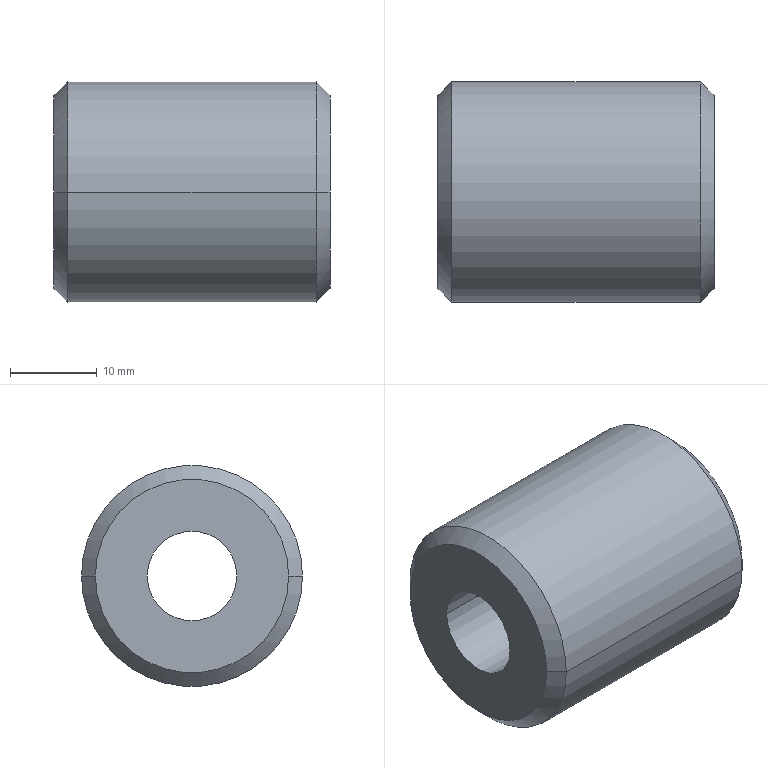Part | NX | features BREP 1 | 1 solid | 10 faces | box 31.75 x 25.4 x 25.4 mm | volume 13243 mm3 | cone 4 | cylinder 4 | plane 2 | commonest cylinder face diameters 10.312 x2 25.4 x2
STEP:
#1=CARTESIAN_POINT('',(-15.875,11.113,0.));
#2=VERTEX_POINT('',#1);
#3=CARTESIAN_POINT('',(-15.875,-11.113,0.));
#4=VERTEX_POINT('',#3);
#5=CARTESIAN_POINT('',(-15.875,0.,0.));
#6=DIRECTION('',(1.,0.,0.));
#7=DIRECTION('',(0.,1.,0.));
#8=AXIS2_PLACEMENT_3D('',#5,#6,#7);
#9=CIRCLE('',#8,11.113);
#10=EDGE_CURVE('',#2,#4,#9,.T.);
#11=ORIENTED_EDGE('',*,*,#10,.F.);
#12=CARTESIAN_POINT('',(-15.875,0.,0.));
#13=DIRECTION('',(1.,0.,0.));
#14=DIRECTION('',(0.,-1.,0.));
#15=AXIS2_PLACEMENT_3D('',#12,#13,#14);
#16=CIRCLE('',#15,11.113);
#17=EDGE_CURVE('',#4,#2,#16,.T.);
#18=ORIENTED_EDGE('',*,*,#17,.F.);
#19=EDGE_LOOP('',(#11,#18));
#20=FACE_BOUND('',#19,.T.);
#21=CARTESIAN_POINT('',(-15.875,5.156,0.));
#22=VERTEX_POINT('',#21);
#23=CARTESIAN_POINT('',(-15.875,-5.156,0.));
#24=VERTEX_POINT('',#23);
#25=CARTESIAN_POINT('',(-15.875,0.,0.));
#26=DIRECTION('',(-1.,0.,0.));
#27=DIRECTION('',(0.,1.,0.));
#28=AXIS2_PLACEMENT_3D('',#25,#26,#27);
#29=CIRCLE('',#28,5.156);
#30=EDGE_CURVE('',#22,#24,#29,.T.);
#31=ORIENTED_EDGE('',*,*,#30,.F.);
#32=CARTESIAN_POINT('',(-15.875,0.,0.));
#33=DIRECTION('',(-1.,0.,0.));
#34=DIRECTION('',(0.,-1.,0.));
#35=AXIS2_PLACEMENT_3D('',#32,#33,#34);
#36=CIRCLE('',#35,5.156);
#37=EDGE_CURVE('',#24,#22,#36,.T.);
#38=ORIENTED_EDGE('',*,*,#37,.F.);
#39=EDGE_LOOP('',(#31,#38));
#40=FACE_BOUND('',#39,.T.);
#41=CARTESIAN_POINT('',(-15.875,0.,0.));
#42=DIRECTION('',(1.,0.,0.));
#43=DIRECTION('',(0.,1.,0.));
#44=AXIS2_PLACEMENT_3D('',#41,#42,#43);
#45=PLANE('',#44);
#46=ADVANCED_FACE('',(#20,#40),#45,.F.);
#47=CARTESIAN_POINT('',(-14.287,12.7,0.));
#48=VERTEX_POINT('',#47);
#49=CARTESIAN_POINT('',(-15.875,11.113,0.));
#50=DIRECTION('',(0.7071,0.7071,0.));
#51=VECTOR('',#50,1000.);
#52=LINE('',#49,#51);
#53=EDGE_CURVE('',#48,#2,#52,.F.);
#54=ORIENTED_EDGE('',*,*,#53,.F.);
#55=CARTESIAN_POINT('',(-14.287,-12.7,0.));
#56=VERTEX_POINT('',#55);
#57=CARTESIAN_POINT('',(-14.287,0.,0.));
#58=DIRECTION('',(1.,0.,0.));
#59=DIRECTION('',(0.,-1.,0.));
#60=AXIS2_PLACEMENT_3D('',#57,#58,#59);
#61=CIRCLE('',#60,12.7);
#62=EDGE_CURVE('',#56,#48,#61,.T.);
#63=ORIENTED_EDGE('',*,*,#62,.F.);
#64=CARTESIAN_POINT('',(-15.875,-11.113,0.));
#65=DIRECTION('',(0.7071,-0.7071,0.));
#66=VECTOR('',#65,1000.);
#67=LINE('',#64,#66);
#68=EDGE_CURVE('',#56,#4,#67,.F.);
#69=ORIENTED_EDGE('',*,*,#68,.T.);
#70=ORIENTED_EDGE('',*,*,#17,.T.);
#71=EDGE_LOOP('',(#54,#63,#69,#70));
#72=FACE_BOUND('',#71,.T.);
#73=CARTESIAN_POINT('',(-15.081,0.,0.));
#74=DIRECTION('',(1.,0.,0.));
#75=DIRECTION('',(0.,-1.,0.));
#76=AXIS2_PLACEMENT_3D('',#73,#74,#75);
#77=CONICAL_SURFACE('',#76,11.906,0.7854);
#78=ADVANCED_FACE('',(#72),#77,.T.);
#79=ORIENTED_EDGE('',*,*,#68,.F.);
#80=CARTESIAN_POINT('',(-14.287,0.,0.));
#81=DIRECTION('',(1.,0.,0.));
#82=DIRECTION('',(0.,1.,0.));
#83=AXIS2_PLACEMENT_3D('',#80,#81,#82);
#84=CIRCLE('',#83,12.7);
#85=EDGE_CURVE('',#48,#56,#84,.T.);
#86=ORIENTED_EDGE('',*,*,#85,.F.);
#87=ORIENTED_EDGE('',*,*,#53,.T.);
#88=ORIENTED_EDGE('',*,*,#10,.T.);
#89=EDGE_LOOP('',(#79,#86,#87,#88));
#90=FACE_BOUND('',#89,.T.);
#91=CARTESIAN_POINT('',(-15.081,0.,0.));
#92=DIRECTION('',(1.,0.,0.));
#93=DIRECTION('',(0.,-1.,0.));
#94=AXIS2_PLACEMENT_3D('',#91,#92,#93);
#95=CONICAL_SURFACE('',#94,11.906,0.7854);
#96=ADVANCED_FACE('',(#90),#95,.T.);
#97=CARTESIAN_POINT('',(14.287,-12.7,0.));
#98=VERTEX_POINT('',#97);
#99=CARTESIAN_POINT('',(-14.287,-12.7,0.));
#100=DIRECTION('',(1.,0.,0.));
#101=VECTOR('',#100,1000.);
#102=LINE('',#99,#101);
#103=EDGE_CURVE('',#56,#98,#102,.T.);
#104=ORIENTED_EDGE('',*,*,#103,.T.);
#105=CARTESIAN_POINT('',(14.287,12.7,0.));
#106=VERTEX_POINT('',#105);
#107=CARTESIAN_POINT('',(14.287,0.,0.));
#108=DIRECTION('',(1.,0.,0.));
#109=DIRECTION('',(0.,1.,0.));
#110=AXIS2_PLACEMENT_3D('',#107,#108,#109);
#111=CIRCLE('',#110,12.7);
#112=EDGE_CURVE('',#106,#98,#111,.T.);
#113=ORIENTED_EDGE('',*,*,#112,.F.);
#114=CARTESIAN_POINT('',(-14.287,12.7,0.));
#115=DIRECTION('',(1.,0.,0.));
#116=VECTOR('',#115,1000.);
#117=LINE('',#114,#116);
#118=EDGE_CURVE('',#48,#106,#117,.T.);
#119=ORIENTED_EDGE('',*,*,#118,.F.);
#120=ORIENTED_EDGE('',*,*,#85,.T.);
#121=EDGE_LOOP('',(#104,#113,#119,#120));
#122=FACE_BOUND('',#121,.T.);
#123=CARTESIAN_POINT('',(-15.875,0.,0.));
#124=DIRECTION('',(1.,0.,0.));
#125=DIRECTION('',(0.,-1.,0.));
#126=AXIS2_PLACEMENT_3D('',#123,#124,#125);
#127=CYLINDRICAL_SURFACE('',#126,12.7);
#128=ADVANCED_FACE('',(#122),#127,.T.);
#129=ORIENTED_EDGE('',*,*,#118,.T.);
#130=CARTESIAN_POINT('',(14.287,0.,0.));
#131=DIRECTION('',(1.,0.,0.));
#132=DIRECTION('',(0.,-1.,0.));
#133=AXIS2_PLACEMENT_3D('',#130,#131,#132);
#134=CIRCLE('',#133,12.7);
#135=EDGE_CURVE('',#98,#106,#134,.T.);
#136=ORIENTED_EDGE('',*,*,#135,.F.);
#137=ORIENTED_EDGE('',*,*,#103,.F.);
#138=ORIENTED_EDGE('',*,*,#62,.T.);
#139=EDGE_LOOP('',(#129,#136,#137,#138));
#140=FACE_BOUND('',#139,.T.);
#141=CARTESIAN_POINT('',(-15.875,0.,0.));
#142=DIRECTION('',(1.,0.,0.));
#143=DIRECTION('',(0.,-1.,0.));
#144=AXIS2_PLACEMENT_3D('',#141,#142,#143);
#145=CYLINDRICAL_SURFACE('',#144,12.7);
#146=ADVANCED_FACE('',(#140),#145,.T.);
#147=CARTESIAN_POINT('',(15.875,-11.113,0.));
#148=VERTEX_POINT('',#147);
#149=CARTESIAN_POINT('',(15.875,-11.113,0.));
#150=DIRECTION('',(-0.7071,-0.7071,0.));
#151=VECTOR('',#150,1000.);
#152=LINE('',#149,#151);
#153=EDGE_CURVE('',#148,#98,#152,.T.);
#154=ORIENTED_EDGE('',*,*,#153,.T.);
#155=ORIENTED_EDGE('',*,*,#135,.T.);
#156=CARTESIAN_POINT('',(15.875,11.113,0.));
#157=VERTEX_POINT('',#156);
#158=CARTESIAN_POINT('',(15.875,11.113,0.));
#159=DIRECTION('',(-0.7071,0.7071,0.));
#160=VECTOR('',#159,1000.);
#161=LINE('',#158,#160);
#162=EDGE_CURVE('',#157,#106,#161,.T.);
#163=ORIENTED_EDGE('',*,*,#162,.F.);
#164=CARTESIAN_POINT('',(15.875,0.,0.));
#165=DIRECTION('',(1.,0.,0.));
#166=DIRECTION('',(0.,-1.,0.));
#167=AXIS2_PLACEMENT_3D('',#164,#165,#166);
#168=CIRCLE('',#167,11.113);
#169=EDGE_CURVE('',#148,#157,#168,.T.);
#170=ORIENTED_EDGE('',*,*,#169,.F.);
#171=EDGE_LOOP('',(#154,#155,#163,#170));
#172=FACE_BOUND('',#171,.T.);
#173=CARTESIAN_POINT('',(15.081,0.,0.));
#174=DIRECTION('',(-1.,0.,0.));
#175=DIRECTION('',(0.,1.,0.));
#176=AXIS2_PLACEMENT_3D('',#173,#174,#175);
#177=CONICAL_SURFACE('',#176,11.906,0.7854);
#178=ADVANCED_FACE('',(#172),#177,.T.);
#179=CARTESIAN_POINT('',(15.875,0.,0.));
#180=DIRECTION('',(1.,0.,0.));
#181=DIRECTION('',(0.,1.,0.));
#182=AXIS2_PLACEMENT_3D('',#179,#180,#181);
#183=CIRCLE('',#182,11.113);
#184=EDGE_CURVE('',#157,#148,#183,.T.);
#185=ORIENTED_EDGE('',*,*,#184,.T.);
#186=ORIENTED_EDGE('',*,*,#169,.T.);
#187=EDGE_LOOP('',(#185,#186));
#188=FACE_BOUND('',#187,.T.);
#189=CARTESIAN_POINT('',(15.875,5.156,0.));
#190=VERTEX_POINT('',#189);
#191=CARTESIAN_POINT('',(15.875,-5.156,0.));
#192=VERTEX_POINT('',#191);
#193=CARTESIAN_POINT('',(15.875,0.,0.));
#194=DIRECTION('',(-1.,0.,0.));
#195=DIRECTION('',(0.,1.,0.));
#196=AXIS2_PLACEMENT_3D('',#193,#194,#195);
#197=CIRCLE('',#196,5.156);
#198=EDGE_CURVE('',#190,#192,#197,.T.);
#199=ORIENTED_EDGE('',*,*,#198,.T.);
#200=CARTESIAN_POINT('',(15.875,0.,0.));
#201=DIRECTION('',(-1.,0.,0.));
#202=DIRECTION('',(0.,-1.,0.));
#203=AXIS2_PLACEMENT_3D('',#200,#201,#202);
#204=CIRCLE('',#203,5.156);
#205=EDGE_CURVE('',#192,#190,#204,.T.);
#206=ORIENTED_EDGE('',*,*,#205,.T.);
#207=EDGE_LOOP('',(#199,#206));
#208=FACE_BOUND('',#207,.T.);
#209=CARTESIAN_POINT('',(15.875,0.,0.));
#210=DIRECTION('',(1.,0.,0.));
#211=DIRECTION('',(0.,1.,0.));
#212=AXIS2_PLACEMENT_3D('',#209,#210,#211);
#213=PLANE('',#212);
#214=ADVANCED_FACE('',(#188,#208),#213,.T.);
#215=ORIENTED_EDGE('',*,*,#162,.T.);
#216=ORIENTED_EDGE('',*,*,#112,.T.);
#217=ORIENTED_EDGE('',*,*,#153,.F.);
#218=ORIENTED_EDGE('',*,*,#184,.F.);
#219=EDGE_LOOP('',(#215,#216,#217,#218));
#220=FACE_BOUND('',#219,.T.);
#221=CARTESIAN_POINT('',(15.081,0.,0.));
#222=DIRECTION('',(-1.,0.,0.));
#223=DIRECTION('',(0.,1.,0.));
#224=AXIS2_PLACEMENT_3D('',#221,#222,#223);
#225=CONICAL_SURFACE('',#224,11.906,0.7854);
#226=ADVANCED_FACE('',(#220),#225,.T.);
#227=CARTESIAN_POINT('',(15.875,5.156,0.));
#228=DIRECTION('',(-1.,0.,0.));
#229=VECTOR('',#228,1000.);
#230=LINE('',#227,#229);
#231=EDGE_CURVE('',#22,#190,#230,.F.);
#232=ORIENTED_EDGE('',*,*,#231,.T.);
#233=ORIENTED_EDGE('',*,*,#205,.F.);
#234=CARTESIAN_POINT('',(15.875,-5.156,0.));
#235=DIRECTION('',(-1.,0.,0.));
#236=VECTOR('',#235,1000.);
#237=LINE('',#234,#236);
#238=EDGE_CURVE('',#24,#192,#237,.F.);
#239=ORIENTED_EDGE('',*,*,#238,.F.);
#240=ORIENTED_EDGE('',*,*,#37,.T.);
#241=EDGE_LOOP('',(#232,#233,#239,#240));
#242=FACE_BOUND('',#241,.T.);
#243=CARTESIAN_POINT('',(15.875,0.,0.));
#244=DIRECTION('',(-1.,0.,0.));
#245=DIRECTION('',(0.,-1.,0.));
#246=AXIS2_PLACEMENT_3D('',#243,#244,#245);
#247=CYLINDRICAL_SURFACE('',#246,5.156);
#248=ADVANCED_FACE('',(#242),#247,.F.);
#249=ORIENTED_EDGE('',*,*,#238,.T.);
#250=ORIENTED_EDGE('',*,*,#198,.F.);
#251=ORIENTED_EDGE('',*,*,#231,.F.);
#252=ORIENTED_EDGE('',*,*,#30,.T.);
#253=EDGE_LOOP('',(#249,#250,#251,#252));
#254=FACE_BOUND('',#253,.T.);
#255=CARTESIAN_POINT('',(15.875,0.,0.));
#256=DIRECTION('',(-1.,0.,0.));
#257=DIRECTION('',(0.,-1.,0.));
#258=AXIS2_PLACEMENT_3D('',#255,#256,#257);
#259=CYLINDRICAL_SURFACE('',#258,5.156);
#260=ADVANCED_FACE('',(#254),#259,.F.);
#261=CLOSED_SHELL('',(#46,#78,#96,#128,#146,#178,#214,#226,#248,#260));
#262=MANIFOLD_SOLID_BREP('',#261);
#263=(LENGTH_UNIT()NAMED_UNIT(*)SI_UNIT(.MILLI.,.METRE.));
#264=UNCERTAINTY_MEASURE_WITH_UNIT(LENGTH_MEASURE(0.00001),#263,'','');
#265=(NAMED_UNIT(*)PLANE_ANGLE_UNIT()SI_UNIT($,.RADIAN.));
#266=(NAMED_UNIT(*)SI_UNIT($,.STERADIAN.)SOLID_ANGLE_UNIT());
#267=(GEOMETRIC_REPRESENTATION_CONTEXT(3)GLOBAL_UNCERTAINTY_ASSIGNED_CONTEXT((#264))GLOBAL_UNIT_ASSIGNED_CONTEXT((#263,#265,#266))REPRESENTATION_CONTEXT('',''));
#268=ADVANCED_BREP_SHAPE_REPRESENTATION('',(#262),#267);